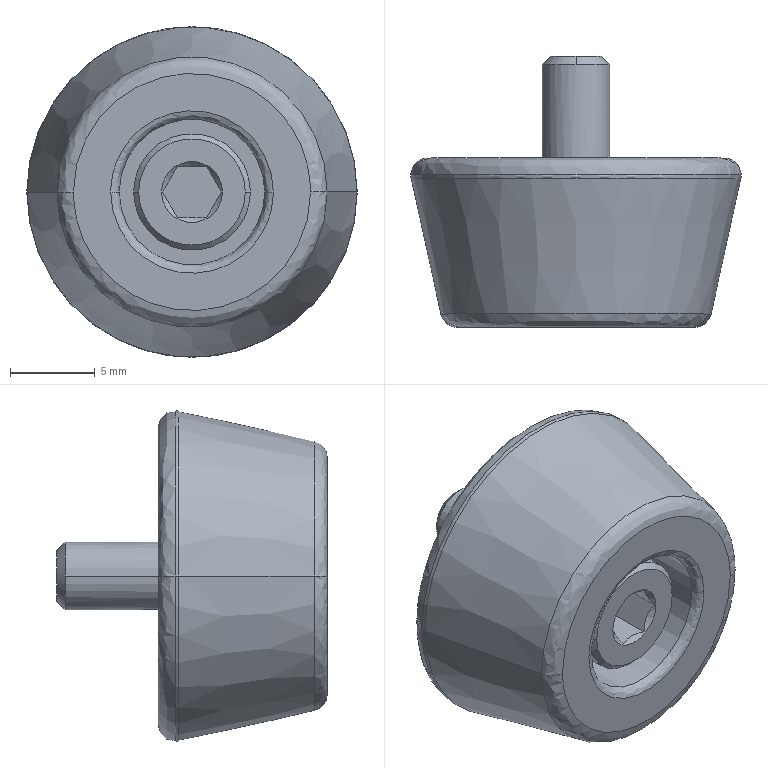Part | SolidWorks | features BaseBody 1 | 1 solid | 34 faces | box 19.513 x 16 x 19.513 mm | volume 2386 mm3 | plane 12 | spline 8 | cone 8 | cylinder 6 | commonest cylinder face diameters 4 x2 6.9 x2 8.6 x2
STEP:
#1=CARTESIAN_POINT('',(9.757,9.,0.));
#2=VERTEX_POINT('',#1);
#3=CARTESIAN_POINT('',(-9.757,9.,0.));
#4=VERTEX_POINT('',#3);
#5=CARTESIAN_POINT('',(0.,9.,0.));
#6=DIRECTION('',(0.,1.,0.));
#7=DIRECTION('',(-1.,0.,0.));
#8=AXIS2_PLACEMENT_3D('',#5,#6,#7);
#9=CIRCLE('',#8,9.757);
#10=EDGE_CURVE('',#2,#4,#9,.T.);
#11=ORIENTED_EDGE('',*,*,#10,.F.);
#12=CARTESIAN_POINT('',(9.733,8.786,0.));
#13=VERTEX_POINT('',#12);
#14=CARTESIAN_POINT('',(8.757,9.,0.));
#15=DIRECTION('',(0.,0.,-1.));
#16=DIRECTION('',(1.,0.,0.));
#17=AXIS2_PLACEMENT_3D('',#14,#15,#16);
#18=CIRCLE('',#17,1.);
#19=EDGE_CURVE('',#2,#13,#18,.T.);
#20=ORIENTED_EDGE('',*,*,#19,.T.);
#21=CARTESIAN_POINT('',(-9.733,8.786,0.));
#22=VERTEX_POINT('',#21);
#23=CARTESIAN_POINT('',(0.,8.786,0.));
#24=DIRECTION('',(0.,1.,0.));
#25=DIRECTION('',(-1.,0.,0.));
#26=AXIS2_PLACEMENT_3D('',#23,#24,#25);
#27=CIRCLE('',#26,9.733);
#28=EDGE_CURVE('',#13,#22,#27,.T.);
#29=ORIENTED_EDGE('',*,*,#28,.T.);
#30=CARTESIAN_POINT('',(-8.757,9.,0.));
#31=DIRECTION('',(0.,0.,1.));
#32=DIRECTION('',(-1.,0.,0.));
#33=AXIS2_PLACEMENT_3D('',#30,#31,#32);
#34=CIRCLE('',#33,1.);
#35=EDGE_CURVE('',#4,#22,#34,.T.);
#36=ORIENTED_EDGE('',*,*,#35,.F.);
#37=EDGE_LOOP('',(#11,#20,#29,#36));
#38=FACE_OUTER_BOUND('',#37,.T.);
#39=CARTESIAN_POINT('',(9.757,9.,0.));
#40=CARTESIAN_POINT('',(9.757,9.,-19.513));
#41=CARTESIAN_POINT('',(-9.757,9.,-19.513));
#42=CARTESIAN_POINT('',(-9.757,9.,0.));
#43=CARTESIAN_POINT('',(9.757,8.928,0.));
#44=CARTESIAN_POINT('',(9.757,8.928,-19.513));
#45=CARTESIAN_POINT('',(-9.757,8.928,-19.513));
#46=CARTESIAN_POINT('',(-9.757,8.928,0.));
#47=CARTESIAN_POINT('',(9.749,8.856,0.));
#48=CARTESIAN_POINT('',(9.749,8.856,-19.498));
#49=CARTESIAN_POINT('',(-9.749,8.856,-19.498));
#50=CARTESIAN_POINT('',(-9.749,8.856,0.));
#51=CARTESIAN_POINT('',(9.733,8.786,0.));
#52=CARTESIAN_POINT('',(9.733,8.786,-19.467));
#53=CARTESIAN_POINT('',(-9.733,8.786,-19.467));
#54=CARTESIAN_POINT('',(-9.733,8.786,0.));
#55=(BOUNDED_SURFACE()B_SPLINE_SURFACE(3,3,((#39,#40,#41,#42),(#43,#44,#45,#46),(#47,#48,#49,#50),(#51,#52,#53,#54)),.UNSPECIFIED.,.F.,.F.,.F.)B_SPLINE_SURFACE_WITH_KNOTS((4,4),(4,4),(0.,1.),(0.,1.),.UNSPECIFIED.)GEOMETRIC_REPRESENTATION_ITEM()RATIONAL_B_SPLINE_SURFACE(((1.,0.3333,0.3333,1.),(0.9961,0.332,0.332,0.9961),(0.9961,0.332,0.332,0.9961),(1.,0.3333,0.3333,1.)))REPRESENTATION_ITEM('')SURFACE());
#56=ADVANCED_FACE('',(#38),#55,.T.);
#57=CARTESIAN_POINT('',(7.977,0.7855,0.));
#58=VERTEX_POINT('',#57);
#59=CARTESIAN_POINT('',(-7.977,0.7855,0.));
#60=VERTEX_POINT('',#59);
#61=CARTESIAN_POINT('',(0.,0.7855,0.));
#62=DIRECTION('',(0.,1.,0.));
#63=DIRECTION('',(-1.,0.,0.));
#64=AXIS2_PLACEMENT_3D('',#61,#62,#63);
#65=CIRCLE('',#64,7.977);
#66=EDGE_CURVE('',#58,#60,#65,.T.);
#67=ORIENTED_EDGE('',*,*,#66,.F.);
#68=CARTESIAN_POINT('',(7.,0.,0.));
#69=VERTEX_POINT('',#68);
#70=CARTESIAN_POINT('',(7.,1.,0.));
#71=DIRECTION('',(0.,0.,-1.));
#72=DIRECTION('',(1.,0.,0.));
#73=AXIS2_PLACEMENT_3D('',#70,#71,#72);
#74=CIRCLE('',#73,1.);
#75=EDGE_CURVE('',#58,#69,#74,.T.);
#76=ORIENTED_EDGE('',*,*,#75,.T.);
#77=CARTESIAN_POINT('',(-7.,0.,0.));
#78=VERTEX_POINT('',#77);
#79=CARTESIAN_POINT('',(7.,0.,0.));
#80=CARTESIAN_POINT('',(7.,0.,-14.));
#81=CARTESIAN_POINT('',(-7.,0.,-14.));
#82=CARTESIAN_POINT('',(-7.,0.,0.));
#83=(BOUNDED_CURVE()B_SPLINE_CURVE(3,(#79,#80,#81,#82),.UNSPECIFIED.,.F.,.F.)B_SPLINE_CURVE_WITH_KNOTS((4,4),(0.,1.),.UNSPECIFIED.)CURVE()GEOMETRIC_REPRESENTATION_ITEM()RATIONAL_B_SPLINE_CURVE((1.,0.3333,0.3333,1.))REPRESENTATION_ITEM(''));
#84=EDGE_CURVE('',#69,#78,#83,.T.);
#85=ORIENTED_EDGE('',*,*,#84,.T.);
#86=CARTESIAN_POINT('',(-7.,1.,0.));
#87=DIRECTION('',(0.,0.,1.));
#88=DIRECTION('',(-1.,0.,0.));
#89=AXIS2_PLACEMENT_3D('',#86,#87,#88);
#90=CIRCLE('',#89,1.);
#91=EDGE_CURVE('',#60,#78,#90,.T.);
#92=ORIENTED_EDGE('',*,*,#91,.F.);
#93=EDGE_LOOP('',(#67,#76,#85,#92));
#94=FACE_OUTER_BOUND('',#93,.T.);
#95=CARTESIAN_POINT('',(7.977,0.7855,0.));
#96=CARTESIAN_POINT('',(7.977,0.7855,-15.953));
#97=CARTESIAN_POINT('',(-7.977,0.7855,-15.953));
#98=CARTESIAN_POINT('',(-7.977,0.7855,0.));
#99=CARTESIAN_POINT('',(7.872,0.307,0.));
#100=CARTESIAN_POINT('',(7.872,0.307,-15.743));
#101=CARTESIAN_POINT('',(-7.872,0.307,-15.743));
#102=CARTESIAN_POINT('',(-7.872,0.307,0.));
#103=CARTESIAN_POINT('',(7.49,0.,0.));
#104=CARTESIAN_POINT('',(7.49,0.,-14.98));
#105=CARTESIAN_POINT('',(-7.49,0.,-14.98));
#106=CARTESIAN_POINT('',(-7.49,0.,0.));
#107=CARTESIAN_POINT('',(7.,0.,0.));
#108=CARTESIAN_POINT('',(7.,0.,-14.));
#109=CARTESIAN_POINT('',(-7.,0.,-14.));
#110=CARTESIAN_POINT('',(-7.,0.,0.));
#111=(BOUNDED_SURFACE()B_SPLINE_SURFACE(3,3,((#95,#96,#97,#98),(#99,#100,#101,#102),(#103,#104,#105,#106),(#107,#108,#109,#110)),.UNSPECIFIED.,.F.,.F.,.F.)B_SPLINE_SURFACE_WITH_KNOTS((4,4),(4,4),(0.,1.),(0.,1.),.UNSPECIFIED.)GEOMETRIC_REPRESENTATION_ITEM()RATIONAL_B_SPLINE_SURFACE(((1.,0.3333,0.3333,1.),(0.8528,0.2843,0.2843,0.8528),(0.8528,0.2843,0.2843,0.8528),(1.,0.3333,0.3333,1.)))REPRESENTATION_ITEM('')SURFACE());
#112=ADVANCED_FACE('',(#94),#111,.T.);
#113=CARTESIAN_POINT('',(-4.8,0.,0.));
#114=VERTEX_POINT('',#113);
#115=CARTESIAN_POINT('',(4.8,0.,0.));
#116=VERTEX_POINT('',#115);
#117=CARTESIAN_POINT('',(-4.8,0.,0.));
#118=CARTESIAN_POINT('',(-4.8,0.,-9.6));
#119=CARTESIAN_POINT('',(4.8,0.,-9.6));
#120=CARTESIAN_POINT('',(4.8,0.,0.));
#121=(BOUNDED_CURVE()B_SPLINE_CURVE(3,(#117,#118,#119,#120),.UNSPECIFIED.,.F.,.F.)B_SPLINE_CURVE_WITH_KNOTS((4,4),(0.,1.),.UNSPECIFIED.)CURVE()GEOMETRIC_REPRESENTATION_ITEM()RATIONAL_B_SPLINE_CURVE((1.,0.3333,0.3333,1.))REPRESENTATION_ITEM(''));
#122=EDGE_CURVE('',#114,#116,#121,.T.);
#123=ORIENTED_EDGE('',*,*,#122,.T.);
#124=CARTESIAN_POINT('',(4.3,0.5,0.));
#125=VERTEX_POINT('',#124);
#126=CARTESIAN_POINT('',(4.8,0.5,0.));
#127=DIRECTION('',(0.,0.,-1.));
#128=DIRECTION('',(1.,0.,0.));
#129=AXIS2_PLACEMENT_3D('',#126,#127,#128);
#130=CIRCLE('',#129,0.5);
#131=EDGE_CURVE('',#116,#125,#130,.T.);
#132=ORIENTED_EDGE('',*,*,#131,.T.);
#133=CARTESIAN_POINT('',(-4.3,0.5,0.));
#134=VERTEX_POINT('',#133);
#135=CARTESIAN_POINT('',(0.,0.5,0.));
#136=DIRECTION('',(0.,1.,0.));
#137=DIRECTION('',(-1.,0.,0.));
#138=AXIS2_PLACEMENT_3D('',#135,#136,#137);
#139=CIRCLE('',#138,4.3);
#140=EDGE_CURVE('',#125,#134,#139,.T.);
#141=ORIENTED_EDGE('',*,*,#140,.T.);
#142=CARTESIAN_POINT('',(-4.8,0.5,0.));
#143=DIRECTION('',(0.,0.,1.));
#144=DIRECTION('',(-1.,0.,0.));
#145=AXIS2_PLACEMENT_3D('',#142,#143,#144);
#146=CIRCLE('',#145,0.5);
#147=EDGE_CURVE('',#114,#134,#146,.T.);
#148=ORIENTED_EDGE('',*,*,#147,.F.);
#149=EDGE_LOOP('',(#123,#132,#141,#148));
#150=FACE_OUTER_BOUND('',#149,.T.);
#151=CARTESIAN_POINT('',(4.8,0.,0.));
#152=CARTESIAN_POINT('',(4.8,0.,-9.6));
#153=CARTESIAN_POINT('',(-4.8,0.,-9.6));
#154=CARTESIAN_POINT('',(-4.8,0.,0.));
#155=CARTESIAN_POINT('',(4.507,0.,0.));
#156=CARTESIAN_POINT('',(4.507,0.,-9.014));
#157=CARTESIAN_POINT('',(-4.507,0.,-9.014));
#158=CARTESIAN_POINT('',(-4.507,0.,0.));
#159=CARTESIAN_POINT('',(4.3,0.2071,0.));
#160=CARTESIAN_POINT('',(4.3,0.2071,-8.6));
#161=CARTESIAN_POINT('',(-4.3,0.2071,-8.6));
#162=CARTESIAN_POINT('',(-4.3,0.2071,0.));
#163=CARTESIAN_POINT('',(4.3,0.5,0.));
#164=CARTESIAN_POINT('',(4.3,0.5,-8.6));
#165=CARTESIAN_POINT('',(-4.3,0.5,-8.6));
#166=CARTESIAN_POINT('',(-4.3,0.5,0.));
#167=(BOUNDED_SURFACE()B_SPLINE_SURFACE(3,3,((#151,#152,#153,#154),(#155,#156,#157,#158),(#159,#160,#161,#162),(#163,#164,#165,#166)),.UNSPECIFIED.,.F.,.F.,.F.)B_SPLINE_SURFACE_WITH_KNOTS((4,4),(4,4),(0.,1.),(0.,1.),.UNSPECIFIED.)GEOMETRIC_REPRESENTATION_ITEM()RATIONAL_B_SPLINE_SURFACE(((1.,0.3333,0.3333,1.),(0.8047,0.2682,0.2682,0.8047),(0.8047,0.2682,0.2682,0.8047),(1.,0.3333,0.3333,1.)))REPRESENTATION_ITEM('')SURFACE());
#168=ADVANCED_FACE('',(#150),#167,.T.);
#169=CARTESIAN_POINT('',(-8.757,10.,0.));
#170=VERTEX_POINT('',#169);
#171=CARTESIAN_POINT('',(8.757,10.,0.));
#172=VERTEX_POINT('',#171);
#173=CARTESIAN_POINT('',(-8.757,10.,0.));
#174=CARTESIAN_POINT('',(-8.757,10.,-17.513));
#175=CARTESIAN_POINT('',(8.757,10.,-17.513));
#176=CARTESIAN_POINT('',(8.757,10.,0.));
#177=(BOUNDED_CURVE()B_SPLINE_CURVE(3,(#173,#174,#175,#176),.UNSPECIFIED.,.F.,.F.)B_SPLINE_CURVE_WITH_KNOTS((4,4),(0.,1.),.UNSPECIFIED.)CURVE()GEOMETRIC_REPRESENTATION_ITEM()RATIONAL_B_SPLINE_CURVE((1.,0.3333,0.3333,1.))REPRESENTATION_ITEM(''));
#178=EDGE_CURVE('',#170,#172,#177,.T.);
#179=ORIENTED_EDGE('',*,*,#178,.T.);
#180=CARTESIAN_POINT('',(8.757,9.,0.));
#181=DIRECTION('',(0.,0.,-1.));
#182=DIRECTION('',(1.,0.,0.));
#183=AXIS2_PLACEMENT_3D('',#180,#181,#182);
#184=CIRCLE('',#183,1.);
#185=EDGE_CURVE('',#172,#2,#184,.T.);
#186=ORIENTED_EDGE('',*,*,#185,.T.);
#187=ORIENTED_EDGE('',*,*,#10,.T.);
#188=CARTESIAN_POINT('',(-8.757,9.,0.));
#189=DIRECTION('',(0.,0.,1.));
#190=DIRECTION('',(-1.,0.,0.));
#191=AXIS2_PLACEMENT_3D('',#188,#189,#190);
#192=CIRCLE('',#191,1.);
#193=EDGE_CURVE('',#170,#4,#192,.T.);
#194=ORIENTED_EDGE('',*,*,#193,.F.);
#195=EDGE_LOOP('',(#179,#186,#187,#194));
#196=FACE_OUTER_BOUND('',#195,.T.);
#197=CARTESIAN_POINT('',(8.757,10.,0.));
#198=CARTESIAN_POINT('',(8.757,10.,-17.513));
#199=CARTESIAN_POINT('',(-8.757,10.,-17.513));
#200=CARTESIAN_POINT('',(-8.757,10.,0.));
#201=CARTESIAN_POINT('',(9.342,10.,0.));
#202=CARTESIAN_POINT('',(9.342,10.,-18.685));
#203=CARTESIAN_POINT('',(-9.342,10.,-18.685));
#204=CARTESIAN_POINT('',(-9.342,10.,0.));
#205=CARTESIAN_POINT('',(9.757,9.586,0.));
#206=CARTESIAN_POINT('',(9.757,9.586,-19.513));
#207=CARTESIAN_POINT('',(-9.757,9.586,-19.513));
#208=CARTESIAN_POINT('',(-9.757,9.586,0.));
#209=CARTESIAN_POINT('',(9.757,9.,0.));
#210=CARTESIAN_POINT('',(9.757,9.,-19.513));
#211=CARTESIAN_POINT('',(-9.757,9.,-19.513));
#212=CARTESIAN_POINT('',(-9.757,9.,0.));
#213=(BOUNDED_SURFACE()B_SPLINE_SURFACE(3,3,((#197,#198,#199,#200),(#201,#202,#203,#204),(#205,#206,#207,#208),(#209,#210,#211,#212)),.UNSPECIFIED.,.F.,.F.,.F.)B_SPLINE_SURFACE_WITH_KNOTS((4,4),(4,4),(0.,1.),(0.,1.),.UNSPECIFIED.)GEOMETRIC_REPRESENTATION_ITEM()RATIONAL_B_SPLINE_SURFACE(((1.,0.3333,0.3333,1.),(0.8047,0.2682,0.2682,0.8047),(0.8047,0.2682,0.2682,0.8047),(1.,0.3333,0.3333,1.)))REPRESENTATION_ITEM('')SURFACE());
#214=ADVANCED_FACE('',(#196),#213,.T.);
#215=ORIENTED_EDGE('',*,*,#185,.F.);
#216=CARTESIAN_POINT('',(8.757,10.,0.));
#217=CARTESIAN_POINT('',(8.757,10.,17.513));
#218=CARTESIAN_POINT('',(-8.757,10.,17.513));
#219=CARTESIAN_POINT('',(-8.757,10.,0.));
#220=(BOUNDED_CURVE()B_SPLINE_CURVE(3,(#216,#217,#218,#219),.UNSPECIFIED.,.F.,.T.)B_SPLINE_CURVE_WITH_KNOTS((4,4),(0.,1.),.UNSPECIFIED.)CURVE()GEOMETRIC_REPRESENTATION_ITEM()RATIONAL_B_SPLINE_CURVE((1.,0.3333,0.3333,1.))REPRESENTATION_ITEM(''));
#221=EDGE_CURVE('',#172,#170,#220,.T.);
#222=ORIENTED_EDGE('',*,*,#221,.T.);
#223=ORIENTED_EDGE('',*,*,#193,.T.);
#224=CARTESIAN_POINT('',(0.,9.,0.));
#225=DIRECTION('',(0.,1.,0.));
#226=DIRECTION('',(-1.,0.,0.));
#227=AXIS2_PLACEMENT_3D('',#224,#225,#226);
#228=CIRCLE('',#227,9.757);
#229=EDGE_CURVE('',#4,#2,#228,.T.);
#230=ORIENTED_EDGE('',*,*,#229,.T.);
#231=EDGE_LOOP('',(#215,#222,#223,#230));
#232=FACE_OUTER_BOUND('',#231,.T.);
#233=CARTESIAN_POINT('',(-8.757,10.,0.));
#234=CARTESIAN_POINT('',(-8.757,10.,17.513));
#235=CARTESIAN_POINT('',(8.757,10.,17.513));
#236=CARTESIAN_POINT('',(8.757,10.,0.));
#237=CARTESIAN_POINT('',(-9.342,10.,0.));
#238=CARTESIAN_POINT('',(-9.342,10.,18.685));
#239=CARTESIAN_POINT('',(9.342,10.,18.685));
#240=CARTESIAN_POINT('',(9.342,10.,0.));
#241=CARTESIAN_POINT('',(-9.757,9.586,0.));
#242=CARTESIAN_POINT('',(-9.757,9.586,19.513));
#243=CARTESIAN_POINT('',(9.757,9.586,19.513));
#244=CARTESIAN_POINT('',(9.757,9.586,0.));
#245=CARTESIAN_POINT('',(-9.757,9.,0.));
#246=CARTESIAN_POINT('',(-9.757,9.,19.513));
#247=CARTESIAN_POINT('',(9.757,9.,19.513));
#248=CARTESIAN_POINT('',(9.757,9.,0.));
#249=(BOUNDED_SURFACE()B_SPLINE_SURFACE(3,3,((#233,#234,#235,#236),(#237,#238,#239,#240),(#241,#242,#243,#244),(#245,#246,#247,#248)),.UNSPECIFIED.,.F.,.F.,.F.)B_SPLINE_SURFACE_WITH_KNOTS((4,4),(4,4),(0.,1.),(0.,1.),.UNSPECIFIED.)GEOMETRIC_REPRESENTATION_ITEM()RATIONAL_B_SPLINE_SURFACE(((1.,0.3333,0.3333,1.),(0.8047,0.2682,0.2682,0.8047),(0.8047,0.2682,0.2682,0.8047),(1.,0.3333,0.3333,1.)))REPRESENTATION_ITEM('')SURFACE());
#250=ADVANCED_FACE('',(#232),#249,.T.);
#251=CARTESIAN_POINT('',(-2.,10.,0.));
#252=VERTEX_POINT('',#251);
#253=CARTESIAN_POINT('',(2.,10.,0.));
#254=VERTEX_POINT('',#253);
#255=CARTESIAN_POINT('',(0.,10.,0.));
#256=DIRECTION('',(0.,1.,0.));
#257=DIRECTION('',(-1.,0.,0.));
#258=AXIS2_PLACEMENT_3D('',#255,#256,#257);
#259=CIRCLE('',#258,2.);
#260=EDGE_CURVE('',#252,#254,#259,.T.);
#261=ORIENTED_EDGE('',*,*,#260,.T.);
#262=CARTESIAN_POINT('',(2.,15.5,0.));
#263=VERTEX_POINT('',#262);
#264=CARTESIAN_POINT('',(2.,16.,0.));
#265=DIRECTION('',(0.,1.,0.));
#266=VECTOR('',#265,1000.);
#267=LINE('',#264,#266);
#268=EDGE_CURVE('',#254,#263,#267,.T.);
#269=ORIENTED_EDGE('',*,*,#268,.T.);
#270=CARTESIAN_POINT('',(0.,15.5,2.));
#271=VERTEX_POINT('',#270);
#272=CARTESIAN_POINT('',(0.,15.5,0.));
#273=DIRECTION('',(0.,-1.,0.));
#274=DIRECTION('',(-1.,0.,0.));
#275=AXIS2_PLACEMENT_3D('',#272,#273,#274);
#276=CIRCLE('',#275,2.);
#277=EDGE_CURVE('',#263,#271,#276,.T.);
#278=ORIENTED_EDGE('',*,*,#277,.T.);
#279=CARTESIAN_POINT('',(-2.,15.5,0.));
#280=VERTEX_POINT('',#279);
#281=CARTESIAN_POINT('',(0.,15.5,0.));
#282=DIRECTION('',(0.,-1.,0.));
#283=DIRECTION('',(-1.,0.,0.));
#284=AXIS2_PLACEMENT_3D('',#281,#282,#283);
#285=CIRCLE('',#284,2.);
#286=EDGE_CURVE('',#271,#280,#285,.T.);
#287=ORIENTED_EDGE('',*,*,#286,.T.);
#288=CARTESIAN_POINT('',(-2.,16.,0.));
#289=DIRECTION('',(0.,1.,0.));
#290=VECTOR('',#289,1000.);
#291=LINE('',#288,#290);
#292=EDGE_CURVE('',#252,#280,#291,.T.);
#293=ORIENTED_EDGE('',*,*,#292,.F.);
#294=EDGE_LOOP('',(#261,#269,#278,#287,#293));
#295=FACE_OUTER_BOUND('',#294,.T.);
#296=CARTESIAN_POINT('',(0.,16.,0.));
#297=DIRECTION('',(0.,1.,0.));
#298=DIRECTION('',(-1.,0.,0.));
#299=AXIS2_PLACEMENT_3D('',#296,#297,#298);
#300=CYLINDRICAL_SURFACE('',#299,2.);
#301=ADVANCED_FACE('',(#295),#300,.T.);
#302=CARTESIAN_POINT('',(0.,0.7855,0.));
#303=DIRECTION('',(0.,1.,0.));
#304=DIRECTION('',(-1.,0.,0.));
#305=AXIS2_PLACEMENT_3D('',#302,#303,#304);
#306=CIRCLE('',#305,7.977);
#307=EDGE_CURVE('',#60,#58,#306,.T.);
#308=ORIENTED_EDGE('',*,*,#307,.T.);
#309=CARTESIAN_POINT('',(9.733,8.786,0.));
#310=DIRECTION('',(0.2145,0.9767,0.));
#311=VECTOR('',#310,1000.);
#312=LINE('',#309,#311);
#313=EDGE_CURVE('',#58,#13,#312,.T.);
#314=ORIENTED_EDGE('',*,*,#313,.T.);
#315=CARTESIAN_POINT('',(0.,8.786,0.));
#316=DIRECTION('',(0.,1.,0.));
#317=DIRECTION('',(-1.,0.,0.));
#318=AXIS2_PLACEMENT_3D('',#315,#316,#317);
#319=CIRCLE('',#318,9.733);
#320=EDGE_CURVE('',#22,#13,#319,.T.);
#321=ORIENTED_EDGE('',*,*,#320,.F.);
#322=CARTESIAN_POINT('',(-9.733,8.786,0.));
#323=DIRECTION('',(-0.2145,0.9767,0.));
#324=VECTOR('',#323,1000.);
#325=LINE('',#322,#324);
#326=EDGE_CURVE('',#60,#22,#325,.T.);
#327=ORIENTED_EDGE('',*,*,#326,.F.);
#328=EDGE_LOOP('',(#308,#314,#321,#327));
#329=FACE_OUTER_BOUND('',#328,.T.);
#330=CARTESIAN_POINT('',(0.,8.786,0.));
#331=DIRECTION('',(0.,1.,0.));
#332=DIRECTION('',(-1.,0.,0.));
#333=AXIS2_PLACEMENT_3D('',#330,#331,#332);
#334=CONICAL_SURFACE('',#333,9.733,0.2161);
#335=ADVANCED_FACE('',(#329),#334,.T.);
#336=CARTESIAN_POINT('',(0.,16.,-1.5));
#337=VERTEX_POINT('',#336);
#338=CARTESIAN_POINT('',(0.,16.,1.5));
#339=VERTEX_POINT('',#338);
#340=CARTESIAN_POINT('',(0.,16.,0.));
#341=DIRECTION('',(0.,-1.,0.));
#342=DIRECTION('',(0.,0.,-1.));
#343=AXIS2_PLACEMENT_3D('',#340,#341,#342);
#344=CIRCLE('',#343,1.5);
#345=EDGE_CURVE('',#337,#339,#344,.T.);
#346=ORIENTED_EDGE('',*,*,#345,.T.);
#347=CARTESIAN_POINT('',(0.,15.5,2.));
#348=DIRECTION('',(0.,-0.7071,0.7071));
#349=VECTOR('',#348,1000.);
#350=LINE('',#347,#349);
#351=EDGE_CURVE('',#339,#271,#350,.T.);
#352=ORIENTED_EDGE('',*,*,#351,.T.);
#353=ORIENTED_EDGE('',*,*,#277,.F.);
#354=CARTESIAN_POINT('',(0.,15.5,-2.));
#355=VERTEX_POINT('',#354);
#356=CARTESIAN_POINT('',(0.,15.5,0.));
#357=DIRECTION('',(0.,-1.,0.));
#358=DIRECTION('',(-1.,0.,0.));
#359=AXIS2_PLACEMENT_3D('',#356,#357,#358);
#360=CIRCLE('',#359,2.);
#361=EDGE_CURVE('',#355,#263,#360,.T.);
#362=ORIENTED_EDGE('',*,*,#361,.F.);
#363=CARTESIAN_POINT('',(0.,15.5,-2.));
#364=DIRECTION('',(0.,-0.7071,-0.7071));
#365=VECTOR('',#364,1000.);
#366=LINE('',#363,#365);
#367=EDGE_CURVE('',#337,#355,#366,.T.);
#368=ORIENTED_EDGE('',*,*,#367,.F.);
#369=EDGE_LOOP('',(#346,#352,#353,#362,#368));
#370=FACE_OUTER_BOUND('',#369,.T.);
#371=CARTESIAN_POINT('',(0.,15.5,0.));
#372=DIRECTION('',(0.,-1.,0.));
#373=DIRECTION('',(0.,0.,-1.));
#374=AXIS2_PLACEMENT_3D('',#371,#372,#373);
#375=CONICAL_SURFACE('',#374,2.,0.7854);
#376=ADVANCED_FACE('',(#370),#375,.T.);
#377=ORIENTED_EDGE('',*,*,#140,.F.);
#378=CARTESIAN_POINT('',(4.3,5.,0.));
#379=VERTEX_POINT('',#378);
#380=CARTESIAN_POINT('',(4.3,16.,0.));
#381=DIRECTION('',(0.,1.,0.));
#382=VECTOR('',#381,1000.);
#383=LINE('',#380,#382);
#384=EDGE_CURVE('',#125,#379,#383,.T.);
#385=ORIENTED_EDGE('',*,*,#384,.T.);
#386=CARTESIAN_POINT('',(-4.3,5.,0.));
#387=VERTEX_POINT('',#386);
#388=CARTESIAN_POINT('',(0.,5.,0.));
#389=DIRECTION('',(0.,-1.,0.));
#390=DIRECTION('',(-1.,0.,0.));
#391=AXIS2_PLACEMENT_3D('',#388,#389,#390);
#392=CIRCLE('',#391,4.3);
#393=EDGE_CURVE('',#387,#379,#392,.T.);
#394=ORIENTED_EDGE('',*,*,#393,.F.);
#395=CARTESIAN_POINT('',(-4.3,16.,0.));
#396=DIRECTION('',(0.,1.,0.));
#397=VECTOR('',#396,1000.);
#398=LINE('',#395,#397);
#399=EDGE_CURVE('',#134,#387,#398,.T.);
#400=ORIENTED_EDGE('',*,*,#399,.F.);
#401=EDGE_LOOP('',(#377,#385,#394,#400));
#402=FACE_OUTER_BOUND('',#401,.T.);
#403=CARTESIAN_POINT('',(0.,16.,0.));
#404=DIRECTION('',(0.,1.,0.));
#405=DIRECTION('',(-1.,0.,0.));
#406=AXIS2_PLACEMENT_3D('',#403,#404,#405);
#407=CYLINDRICAL_SURFACE('',#406,4.3);
#408=ADVANCED_FACE('',(#402),#407,.F.);
#409=CARTESIAN_POINT('',(-3.45,1.3,0.));
#410=VERTEX_POINT('',#409);
#411=CARTESIAN_POINT('',(3.45,1.3,0.));
#412=VERTEX_POINT('',#411);
#413=CARTESIAN_POINT('',(0.,1.3,0.));
#414=DIRECTION('',(0.,1.,0.));
#415=DIRECTION('',(-1.,0.,0.));
#416=AXIS2_PLACEMENT_3D('',#413,#414,#415);
#417=CIRCLE('',#416,3.45);
#418=EDGE_CURVE('',#410,#412,#417,.T.);
#419=ORIENTED_EDGE('',*,*,#418,.T.);
#420=CARTESIAN_POINT('',(3.45,5.,0.));
#421=VERTEX_POINT('',#420);
#422=CARTESIAN_POINT('',(3.45,16.,0.));
#423=DIRECTION('',(0.,1.,0.));
#424=VECTOR('',#423,1000.);
#425=LINE('',#422,#424);
#426=EDGE_CURVE('',#412,#421,#425,.T.);
#427=ORIENTED_EDGE('',*,*,#426,.T.);
#428=CARTESIAN_POINT('',(-3.45,5.,0.));
#429=VERTEX_POINT('',#428);
#430=CARTESIAN_POINT('',(0.,5.,0.));
#431=DIRECTION('',(0.,-1.,0.));
#432=DIRECTION('',(-1.,0.,0.));
#433=AXIS2_PLACEMENT_3D('',#430,#431,#432);
#434=CIRCLE('',#433,3.45);
#435=EDGE_CURVE('',#421,#429,#434,.T.);
#436=ORIENTED_EDGE('',*,*,#435,.T.);
#437=CARTESIAN_POINT('',(-3.45,16.,0.));
#438=DIRECTION('',(0.,1.,0.));
#439=VECTOR('',#438,1000.);
#440=LINE('',#437,#439);
#441=EDGE_CURVE('',#410,#429,#440,.T.);
#442=ORIENTED_EDGE('',*,*,#441,.F.);
#443=EDGE_LOOP('',(#419,#427,#436,#442));
#444=FACE_OUTER_BOUND('',#443,.T.);
#445=CARTESIAN_POINT('',(0.,16.,0.));
#446=DIRECTION('',(0.,1.,0.));
#447=DIRECTION('',(-1.,0.,0.));
#448=AXIS2_PLACEMENT_3D('',#445,#446,#447);
#449=CYLINDRICAL_SURFACE('',#448,3.45);
#450=ADVANCED_FACE('',(#444),#449,.T.);
#451=CARTESIAN_POINT('',(-3.15,1.,0.));
#452=VERTEX_POINT('',#451);
#453=CARTESIAN_POINT('',(3.15,1.,0.));
#454=VERTEX_POINT('',#453);
#455=CARTESIAN_POINT('',(0.,1.,0.));
#456=DIRECTION('',(0.,1.,0.));
#457=DIRECTION('',(-1.,0.,0.));
#458=AXIS2_PLACEMENT_3D('',#455,#456,#457);
#459=CIRCLE('',#458,3.15);
#460=EDGE_CURVE('',#452,#454,#459,.T.);
#461=ORIENTED_EDGE('',*,*,#460,.T.);
#462=CARTESIAN_POINT('',(3.45,1.3,0.));
#463=DIRECTION('',(0.7071,0.7071,0.));
#464=VECTOR('',#463,1000.);
#465=LINE('',#462,#464);
#466=EDGE_CURVE('',#454,#412,#465,.T.);
#467=ORIENTED_EDGE('',*,*,#466,.T.);
#468=ORIENTED_EDGE('',*,*,#418,.F.);
#469=CARTESIAN_POINT('',(-3.45,1.3,0.));
#470=DIRECTION('',(-0.7071,0.7071,0.));
#471=VECTOR('',#470,1000.);
#472=LINE('',#469,#471);
#473=EDGE_CURVE('',#452,#410,#472,.T.);
#474=ORIENTED_EDGE('',*,*,#473,.F.);
#475=EDGE_LOOP('',(#461,#467,#468,#474));
#476=FACE_OUTER_BOUND('',#475,.T.);
#477=CARTESIAN_POINT('',(0.,1.3,0.));
#478=DIRECTION('',(0.,1.,0.));
#479=DIRECTION('',(-1.,0.,0.));
#480=AXIS2_PLACEMENT_3D('',#477,#478,#479);
#481=CONICAL_SURFACE('',#480,3.45,0.7854);
#482=ADVANCED_FACE('',(#476),#481,.T.);
#483=CARTESIAN_POINT('',(-1.732,1.068,0.));
#484=VERTEX_POINT('',#483);
#485=CARTESIAN_POINT('',(-0.866,1.068,-1.5));
#486=VERTEX_POINT('',#485);
#487=CARTESIAN_POINT('',(-1.732,1.068,0.));
#488=CARTESIAN_POINT('',(-1.664,1.136,-0.1172));
#489=CARTESIAN_POINT('',(-1.595,1.193,-0.237));
#490=CARTESIAN_POINT('',(-1.452,1.275,-0.4853));
#491=CARTESIAN_POINT('',(-1.376,1.3,-0.6163));
#492=CARTESIAN_POINT('',(-1.149,1.301,-1.009));
#493=CARTESIAN_POINT('',(-1.002,1.204,-1.264));
#494=CARTESIAN_POINT('',(-0.866,1.068,-1.5));
#495=B_SPLINE_CURVE_WITH_KNOTS('',3,(#487,#488,#489,#490,#491,#492,#493,#494),.UNSPECIFIED.,.F.,.F.,(4,2,2,4),(0.,0.0004473,0.0008946,0.001789),.UNSPECIFIED.);
#496=EDGE_CURVE('',#484,#486,#495,.T.);
#497=ORIENTED_EDGE('',*,*,#496,.F.);
#498=CARTESIAN_POINT('',(-1.8,1.,0.));
#499=VERTEX_POINT('',#498);
#500=CARTESIAN_POINT('',(-1.8,1.,0.));
#501=DIRECTION('',(-0.7071,-0.7071,0.));
#502=VECTOR('',#501,1000.);
#503=LINE('',#500,#502);
#504=EDGE_CURVE('',#484,#499,#503,.T.);
#505=ORIENTED_EDGE('',*,*,#504,.T.);
#506=CARTESIAN_POINT('',(1.8,1.,0.));
#507=VERTEX_POINT('',#506);
#508=CARTESIAN_POINT('',(0.,1.,0.));
#509=DIRECTION('',(0.,-1.,0.));
#510=DIRECTION('',(1.,0.,0.));
#511=AXIS2_PLACEMENT_3D('',#508,#509,#510);
#512=CIRCLE('',#511,1.8);
#513=EDGE_CURVE('',#499,#507,#512,.T.);
#514=ORIENTED_EDGE('',*,*,#513,.T.);
#515=CARTESIAN_POINT('',(1.732,1.068,0.));
#516=VERTEX_POINT('',#515);
#517=CARTESIAN_POINT('',(1.8,1.,0.));
#518=DIRECTION('',(0.7071,-0.7071,0.));
#519=VECTOR('',#518,1000.);
#520=LINE('',#517,#519);
#521=EDGE_CURVE('',#516,#507,#520,.T.);
#522=ORIENTED_EDGE('',*,*,#521,.F.);
#523=CARTESIAN_POINT('',(0.866,1.068,-1.5));
#524=VERTEX_POINT('',#523);
#525=CARTESIAN_POINT('',(0.866,1.068,-1.5));
#526=CARTESIAN_POINT('',(0.9337,1.136,-1.383));
#527=CARTESIAN_POINT('',(1.003,1.193,-1.263));
#528=CARTESIAN_POINT('',(1.146,1.275,-1.015));
#529=CARTESIAN_POINT('',(1.222,1.3,-0.8837));
#530=CARTESIAN_POINT('',(1.449,1.301,-0.4909));
#531=CARTESIAN_POINT('',(1.596,1.204,-0.2358));
#532=CARTESIAN_POINT('',(1.732,1.068,0.));
#533=B_SPLINE_CURVE_WITH_KNOTS('',3,(#525,#526,#527,#528,#529,#530,#531,#532),.UNSPECIFIED.,.F.,.F.,(4,2,2,4),(0.,0.0004473,0.0008946,0.001789),.UNSPECIFIED.);
#534=EDGE_CURVE('',#524,#516,#533,.T.);
#535=ORIENTED_EDGE('',*,*,#534,.F.);
#536=CARTESIAN_POINT('',(-0.866,1.068,-1.5));
#537=CARTESIAN_POINT('',(-0.7307,1.136,-1.5));
#538=CARTESIAN_POINT('',(-0.5923,1.193,-1.5));
#539=CARTESIAN_POINT('',(-0.3056,1.275,-1.5));
#540=CARTESIAN_POINT('',(-0.1544,1.3,-1.5));
#541=CARTESIAN_POINT('',(0.2992,1.301,-1.5));
#542=CARTESIAN_POINT('',(0.5938,1.204,-1.5));
#543=CARTESIAN_POINT('',(0.866,1.068,-1.5));
#544=B_SPLINE_CURVE_WITH_KNOTS('',3,(#536,#537,#538,#539,#540,#541,#542,#543),.UNSPECIFIED.,.F.,.F.,(4,2,2,4),(0.,0.0004473,0.0008946,0.001789),.UNSPECIFIED.);
#545=EDGE_CURVE('',#486,#524,#544,.T.);
#546=ORIENTED_EDGE('',*,*,#545,.F.);
#547=EDGE_LOOP('',(#497,#505,#514,#522,#535,#546));
#548=FACE_OUTER_BOUND('',#547,.T.);
#549=CARTESIAN_POINT('',(0.,1.,0.));
#550=DIRECTION('',(0.,-1.,0.));
#551=DIRECTION('',(1.,0.,0.));
#552=AXIS2_PLACEMENT_3D('',#549,#550,#551);
#553=CONICAL_SURFACE('',#552,1.8,0.7854);
#554=ADVANCED_FACE('',(#548),#553,.F.);
#555=ORIENTED_EDGE('',*,*,#178,.F.);
#556=ORIENTED_EDGE('',*,*,#221,.F.);
#557=EDGE_LOOP('',(#555,#556));
#558=FACE_OUTER_BOUND('',#557,.T.);
#559=ORIENTED_EDGE('',*,*,#260,.F.);
#560=CARTESIAN_POINT('',(0.,10.,0.));
#561=DIRECTION('',(0.,1.,0.));
#562=DIRECTION('',(-1.,0.,0.));
#563=AXIS2_PLACEMENT_3D('',#560,#561,#562);
#564=CIRCLE('',#563,2.);
#565=EDGE_CURVE('',#254,#252,#564,.T.);
#566=ORIENTED_EDGE('',*,*,#565,.F.);
#567=EDGE_LOOP('',(#559,#566));
#568=FACE_BOUND('',#567,.T.);
#569=CARTESIAN_POINT('',(8.757,10.,0.));
#570=DIRECTION('',(0.,-1.,0.));
#571=DIRECTION('',(1.,0.,0.));
#572=AXIS2_PLACEMENT_3D('',#569,#570,#571);
#573=PLANE('',#572);
#574=ADVANCED_FACE('',(#558,#568),#573,.F.);
#575=ORIENTED_EDGE('',*,*,#19,.F.);
#576=ORIENTED_EDGE('',*,*,#229,.F.);
#577=ORIENTED_EDGE('',*,*,#35,.T.);
#578=ORIENTED_EDGE('',*,*,#320,.T.);
#579=EDGE_LOOP('',(#575,#576,#577,#578));
#580=FACE_OUTER_BOUND('',#579,.T.);
#581=CARTESIAN_POINT('',(-9.757,9.,0.));
#582=CARTESIAN_POINT('',(-9.757,9.,19.513));
#583=CARTESIAN_POINT('',(9.757,9.,19.513));
#584=CARTESIAN_POINT('',(9.757,9.,0.));
#585=CARTESIAN_POINT('',(-9.757,8.928,0.));
#586=CARTESIAN_POINT('',(-9.757,8.928,19.513));
#587=CARTESIAN_POINT('',(9.757,8.928,19.513));
#588=CARTESIAN_POINT('',(9.757,8.928,0.));
#589=CARTESIAN_POINT('',(-9.749,8.856,0.));
#590=CARTESIAN_POINT('',(-9.749,8.856,19.498));
#591=CARTESIAN_POINT('',(9.749,8.856,19.498));
#592=CARTESIAN_POINT('',(9.749,8.856,0.));
#593=CARTESIAN_POINT('',(-9.733,8.786,0.));
#594=CARTESIAN_POINT('',(-9.733,8.786,19.467));
#595=CARTESIAN_POINT('',(9.733,8.786,19.467));
#596=CARTESIAN_POINT('',(9.733,8.786,0.));
#597=(BOUNDED_SURFACE()B_SPLINE_SURFACE(3,3,((#581,#582,#583,#584),(#585,#586,#587,#588),(#589,#590,#591,#592),(#593,#594,#595,#596)),.UNSPECIFIED.,.F.,.F.,.F.)B_SPLINE_SURFACE_WITH_KNOTS((4,4),(4,4),(0.,1.),(0.,1.),.UNSPECIFIED.)GEOMETRIC_REPRESENTATION_ITEM()RATIONAL_B_SPLINE_SURFACE(((1.,0.3333,0.3333,1.),(0.9961,0.332,0.332,0.9961),(0.9961,0.332,0.332,0.9961),(1.,0.3333,0.3333,1.)))REPRESENTATION_ITEM('')SURFACE());
#598=ADVANCED_FACE('',(#580),#597,.T.);
#599=ORIENTED_EDGE('',*,*,#268,.F.);
#600=ORIENTED_EDGE('',*,*,#565,.T.);
#601=ORIENTED_EDGE('',*,*,#292,.T.);
#602=CARTESIAN_POINT('',(0.,15.5,0.));
#603=DIRECTION('',(0.,-1.,0.));
#604=DIRECTION('',(-1.,0.,0.));
#605=AXIS2_PLACEMENT_3D('',#602,#603,#604);
#606=CIRCLE('',#605,2.);
#607=EDGE_CURVE('',#280,#355,#606,.T.);
#608=ORIENTED_EDGE('',*,*,#607,.T.);
#609=ORIENTED_EDGE('',*,*,#361,.T.);
#610=EDGE_LOOP('',(#599,#600,#601,#608,#609));
#611=FACE_OUTER_BOUND('',#610,.T.);
#612=CARTESIAN_POINT('',(0.,16.,0.));
#613=DIRECTION('',(0.,1.,0.));
#614=DIRECTION('',(-1.,0.,0.));
#615=AXIS2_PLACEMENT_3D('',#612,#613,#614);
#616=CYLINDRICAL_SURFACE('',#615,2.);
#617=ADVANCED_FACE('',(#611),#616,.T.);
#618=ORIENTED_EDGE('',*,*,#313,.F.);
#619=ORIENTED_EDGE('',*,*,#66,.T.);
#620=ORIENTED_EDGE('',*,*,#326,.T.);
#621=ORIENTED_EDGE('',*,*,#28,.F.);
#622=EDGE_LOOP('',(#618,#619,#620,#621));
#623=FACE_OUTER_BOUND('',#622,.T.);
#624=CARTESIAN_POINT('',(0.,8.786,0.));
#625=DIRECTION('',(0.,1.,0.));
#626=DIRECTION('',(-1.,0.,0.));
#627=AXIS2_PLACEMENT_3D('',#624,#625,#626);
#628=CONICAL_SURFACE('',#627,9.733,0.2161);
#629=ADVANCED_FACE('',(#623),#628,.T.);
#630=ORIENTED_EDGE('',*,*,#351,.F.);
#631=CARTESIAN_POINT('',(0.,16.,0.));
#632=DIRECTION('',(0.,-1.,0.));
#633=DIRECTION('',(0.,0.,-1.));
#634=AXIS2_PLACEMENT_3D('',#631,#632,#633);
#635=CIRCLE('',#634,1.5);
#636=EDGE_CURVE('',#339,#337,#635,.T.);
#637=ORIENTED_EDGE('',*,*,#636,.T.);
#638=ORIENTED_EDGE('',*,*,#367,.T.);
#639=ORIENTED_EDGE('',*,*,#607,.F.);
#640=ORIENTED_EDGE('',*,*,#286,.F.);
#641=EDGE_LOOP('',(#630,#637,#638,#639,#640));
#642=FACE_OUTER_BOUND('',#641,.T.);
#643=CARTESIAN_POINT('',(0.,15.5,0.));
#644=DIRECTION('',(0.,-1.,0.));
#645=DIRECTION('',(0.,0.,-1.));
#646=AXIS2_PLACEMENT_3D('',#643,#644,#645);
#647=CONICAL_SURFACE('',#646,2.,0.7854);
#648=ADVANCED_FACE('',(#642),#647,.T.);
#649=ORIENTED_EDGE('',*,*,#75,.F.);
#650=ORIENTED_EDGE('',*,*,#307,.F.);
#651=ORIENTED_EDGE('',*,*,#91,.T.);
#652=CARTESIAN_POINT('',(-7.,0.,0.));
#653=CARTESIAN_POINT('',(-7.,0.,14.));
#654=CARTESIAN_POINT('',(7.,0.,14.));
#655=CARTESIAN_POINT('',(7.,0.,0.));
#656=(BOUNDED_CURVE()B_SPLINE_CURVE(3,(#652,#653,#654,#655),.UNSPECIFIED.,.F.,.F.)B_SPLINE_CURVE_WITH_KNOTS((4,4),(0.,1.),.UNSPECIFIED.)CURVE()GEOMETRIC_REPRESENTATION_ITEM()RATIONAL_B_SPLINE_CURVE((1.,0.3333,0.3333,1.))REPRESENTATION_ITEM(''));
#657=EDGE_CURVE('',#78,#69,#656,.T.);
#658=ORIENTED_EDGE('',*,*,#657,.T.);
#659=EDGE_LOOP('',(#649,#650,#651,#658));
#660=FACE_OUTER_BOUND('',#659,.T.);
#661=CARTESIAN_POINT('',(-7.977,0.7855,0.));
#662=CARTESIAN_POINT('',(-7.977,0.7855,15.953));
#663=CARTESIAN_POINT('',(7.977,0.7855,15.953));
#664=CARTESIAN_POINT('',(7.977,0.7855,0.));
#665=CARTESIAN_POINT('',(-7.872,0.307,0.));
#666=CARTESIAN_POINT('',(-7.872,0.307,15.743));
#667=CARTESIAN_POINT('',(7.872,0.307,15.743));
#668=CARTESIAN_POINT('',(7.872,0.307,0.));
#669=CARTESIAN_POINT('',(-7.49,0.,0.));
#670=CARTESIAN_POINT('',(-7.49,0.,14.98));
#671=CARTESIAN_POINT('',(7.49,0.,14.98));
#672=CARTESIAN_POINT('',(7.49,0.,0.));
#673=CARTESIAN_POINT('',(-7.,0.,0.));
#674=CARTESIAN_POINT('',(-7.,0.,14.));
#675=CARTESIAN_POINT('',(7.,0.,14.));
#676=CARTESIAN_POINT('',(7.,0.,0.));
#677=(BOUNDED_SURFACE()B_SPLINE_SURFACE(3,3,((#661,#662,#663,#664),(#665,#666,#667,#668),(#669,#670,#671,#672),(#673,#674,#675,#676)),.UNSPECIFIED.,.F.,.F.,.F.)B_SPLINE_SURFACE_WITH_KNOTS((4,4),(4,4),(0.,1.),(0.,1.),.UNSPECIFIED.)GEOMETRIC_REPRESENTATION_ITEM()RATIONAL_B_SPLINE_SURFACE(((1.,0.3333,0.3333,1.),(0.8528,0.2843,0.2843,0.8528),(0.8528,0.2843,0.2843,0.8528),(1.,0.3333,0.3333,1.)))REPRESENTATION_ITEM('')SURFACE());
#678=ADVANCED_FACE('',(#660),#677,.T.);
#679=ORIENTED_EDGE('',*,*,#345,.F.);
#680=ORIENTED_EDGE('',*,*,#636,.F.);
#681=EDGE_LOOP('',(#679,#680));
#682=FACE_OUTER_BOUND('',#681,.T.);
#683=CARTESIAN_POINT('',(2.,16.,0.));
#684=DIRECTION('',(0.,-1.,0.));
#685=DIRECTION('',(1.,0.,0.));
#686=AXIS2_PLACEMENT_3D('',#683,#684,#685);
#687=PLANE('',#686);
#688=ADVANCED_FACE('',(#682),#687,.F.);
#689=ORIENTED_EDGE('',*,*,#84,.F.);
#690=ORIENTED_EDGE('',*,*,#657,.F.);
#691=EDGE_LOOP('',(#689,#690));
#692=FACE_OUTER_BOUND('',#691,.T.);
#693=ORIENTED_EDGE('',*,*,#122,.F.);
#694=CARTESIAN_POINT('',(4.8,0.,0.));
#695=CARTESIAN_POINT('',(4.8,0.,9.6));
#696=CARTESIAN_POINT('',(-4.8,0.,9.6));
#697=CARTESIAN_POINT('',(-4.8,0.,0.));
#698=(BOUNDED_CURVE()B_SPLINE_CURVE(3,(#694,#695,#696,#697),.UNSPECIFIED.,.F.,.F.)B_SPLINE_CURVE_WITH_KNOTS((4,4),(0.,1.),.UNSPECIFIED.)CURVE()GEOMETRIC_REPRESENTATION_ITEM()RATIONAL_B_SPLINE_CURVE((1.,0.3333,0.3333,1.))REPRESENTATION_ITEM(''));
#699=EDGE_CURVE('',#116,#114,#698,.T.);
#700=ORIENTED_EDGE('',*,*,#699,.F.);
#701=EDGE_LOOP('',(#693,#700));
#702=FACE_BOUND('',#701,.T.);
#703=CARTESIAN_POINT('',(4.3,0.,0.));
#704=DIRECTION('',(0.,1.,0.));
#705=DIRECTION('',(-1.,0.,0.));
#706=AXIS2_PLACEMENT_3D('',#703,#704,#705);
#707=PLANE('',#706);
#708=ADVANCED_FACE('',(#692,#702),#707,.F.);
#709=ORIENTED_EDGE('',*,*,#131,.F.);
#710=ORIENTED_EDGE('',*,*,#699,.T.);
#711=ORIENTED_EDGE('',*,*,#147,.T.);
#712=CARTESIAN_POINT('',(0.,0.5,0.));
#713=DIRECTION('',(0.,1.,0.));
#714=DIRECTION('',(-1.,0.,0.));
#715=AXIS2_PLACEMENT_3D('',#712,#713,#714);
#716=CIRCLE('',#715,4.3);
#717=EDGE_CURVE('',#134,#125,#716,.T.);
#718=ORIENTED_EDGE('',*,*,#717,.T.);
#719=EDGE_LOOP('',(#709,#710,#711,#718));
#720=FACE_OUTER_BOUND('',#719,.T.);
#721=CARTESIAN_POINT('',(-4.8,0.,0.));
#722=CARTESIAN_POINT('',(-4.8,0.,9.6));
#723=CARTESIAN_POINT('',(4.8,0.,9.6));
#724=CARTESIAN_POINT('',(4.8,0.,0.));
#725=CARTESIAN_POINT('',(-4.507,0.,0.));
#726=CARTESIAN_POINT('',(-4.507,0.,9.014));
#727=CARTESIAN_POINT('',(4.507,0.,9.014));
#728=CARTESIAN_POINT('',(4.507,0.,0.));
#729=CARTESIAN_POINT('',(-4.3,0.2071,0.));
#730=CARTESIAN_POINT('',(-4.3,0.2071,8.6));
#731=CARTESIAN_POINT('',(4.3,0.2071,8.6));
#732=CARTESIAN_POINT('',(4.3,0.2071,0.));
#733=CARTESIAN_POINT('',(-4.3,0.5,0.));
#734=CARTESIAN_POINT('',(-4.3,0.5,8.6));
#735=CARTESIAN_POINT('',(4.3,0.5,8.6));
#736=CARTESIAN_POINT('',(4.3,0.5,0.));
#737=(BOUNDED_SURFACE()B_SPLINE_SURFACE(3,3,((#721,#722,#723,#724),(#725,#726,#727,#728),(#729,#730,#731,#732),(#733,#734,#735,#736)),.UNSPECIFIED.,.F.,.F.,.F.)B_SPLINE_SURFACE_WITH_KNOTS((4,4),(4,4),(0.,1.),(0.,1.),.UNSPECIFIED.)GEOMETRIC_REPRESENTATION_ITEM()RATIONAL_B_SPLINE_SURFACE(((1.,0.3333,0.3333,1.),(0.8047,0.2682,0.2682,0.8047),(0.8047,0.2682,0.2682,0.8047),(1.,0.3333,0.3333,1.)))REPRESENTATION_ITEM('')SURFACE());
#738=ADVANCED_FACE('',(#720),#737,.T.);
#739=ORIENTED_EDGE('',*,*,#384,.F.);
#740=ORIENTED_EDGE('',*,*,#717,.F.);
#741=ORIENTED_EDGE('',*,*,#399,.T.);
#742=CARTESIAN_POINT('',(0.,5.,0.));
#743=DIRECTION('',(0.,-1.,0.));
#744=DIRECTION('',(-1.,0.,0.));
#745=AXIS2_PLACEMENT_3D('',#742,#743,#744);
#746=CIRCLE('',#745,4.3);
#747=EDGE_CURVE('',#379,#387,#746,.T.);
#748=ORIENTED_EDGE('',*,*,#747,.F.);
#749=EDGE_LOOP('',(#739,#740,#741,#748));
#750=FACE_OUTER_BOUND('',#749,.T.);
#751=CARTESIAN_POINT('',(0.,16.,0.));
#752=DIRECTION('',(0.,1.,0.));
#753=DIRECTION('',(-1.,0.,0.));
#754=AXIS2_PLACEMENT_3D('',#751,#752,#753);
#755=CYLINDRICAL_SURFACE('',#754,4.3);
#756=ADVANCED_FACE('',(#750),#755,.F.);
#757=CARTESIAN_POINT('',(0.,5.,0.));
#758=DIRECTION('',(0.,-1.,0.));
#759=DIRECTION('',(-1.,0.,0.));
#760=AXIS2_PLACEMENT_3D('',#757,#758,#759);
#761=CIRCLE('',#760,3.45);
#762=EDGE_CURVE('',#429,#421,#761,.T.);
#763=ORIENTED_EDGE('',*,*,#762,.F.);
#764=ORIENTED_EDGE('',*,*,#435,.F.);
#765=EDGE_LOOP('',(#763,#764));
#766=FACE_BOUND('',#765,.T.);
#767=ORIENTED_EDGE('',*,*,#393,.T.);
#768=ORIENTED_EDGE('',*,*,#747,.T.);
#769=EDGE_LOOP('',(#767,#768));
#770=FACE_OUTER_BOUND('',#769,.T.);
#771=CARTESIAN_POINT('',(3.45,5.,0.));
#772=DIRECTION('',(0.,1.,0.));
#773=DIRECTION('',(-1.,0.,0.));
#774=AXIS2_PLACEMENT_3D('',#771,#772,#773);
#775=PLANE('',#774);
#776=ADVANCED_FACE('',(#766,#770),#775,.F.);
#777=ORIENTED_EDGE('',*,*,#426,.F.);
#778=CARTESIAN_POINT('',(0.,1.3,0.));
#779=DIRECTION('',(0.,1.,0.));
#780=DIRECTION('',(-1.,0.,0.));
#781=AXIS2_PLACEMENT_3D('',#778,#779,#780);
#782=CIRCLE('',#781,3.45);
#783=EDGE_CURVE('',#412,#410,#782,.T.);
#784=ORIENTED_EDGE('',*,*,#783,.T.);
#785=ORIENTED_EDGE('',*,*,#441,.T.);
#786=ORIENTED_EDGE('',*,*,#762,.T.);
#787=EDGE_LOOP('',(#777,#784,#785,#786));
#788=FACE_OUTER_BOUND('',#787,.T.);
#789=CARTESIAN_POINT('',(0.,16.,0.));
#790=DIRECTION('',(0.,1.,0.));
#791=DIRECTION('',(-1.,0.,0.));
#792=AXIS2_PLACEMENT_3D('',#789,#790,#791);
#793=CYLINDRICAL_SURFACE('',#792,3.45);
#794=ADVANCED_FACE('',(#788),#793,.T.);
#795=ORIENTED_EDGE('',*,*,#466,.F.);
#796=CARTESIAN_POINT('',(0.,1.,0.));
#797=DIRECTION('',(0.,1.,0.));
#798=DIRECTION('',(-1.,0.,0.));
#799=AXIS2_PLACEMENT_3D('',#796,#797,#798);
#800=CIRCLE('',#799,3.15);
#801=EDGE_CURVE('',#454,#452,#800,.T.);
#802=ORIENTED_EDGE('',*,*,#801,.T.);
#803=ORIENTED_EDGE('',*,*,#473,.T.);
#804=ORIENTED_EDGE('',*,*,#783,.F.);
#805=EDGE_LOOP('',(#795,#802,#803,#804));
#806=FACE_OUTER_BOUND('',#805,.T.);
#807=CARTESIAN_POINT('',(0.,1.3,0.));
#808=DIRECTION('',(0.,1.,0.));
#809=DIRECTION('',(-1.,0.,0.));
#810=AXIS2_PLACEMENT_3D('',#807,#808,#809);
#811=CONICAL_SURFACE('',#810,3.45,0.7854);
#812=ADVANCED_FACE('',(#806),#811,.T.);
#813=CARTESIAN_POINT('',(0.,1.,0.));
#814=DIRECTION('',(0.,-1.,0.));
#815=DIRECTION('',(1.,0.,0.));
#816=AXIS2_PLACEMENT_3D('',#813,#814,#815);
#817=CIRCLE('',#816,1.8);
#818=EDGE_CURVE('',#507,#499,#817,.T.);
#819=ORIENTED_EDGE('',*,*,#818,.F.);
#820=ORIENTED_EDGE('',*,*,#513,.F.);
#821=EDGE_LOOP('',(#819,#820));
#822=FACE_BOUND('',#821,.T.);
#823=ORIENTED_EDGE('',*,*,#460,.F.);
#824=ORIENTED_EDGE('',*,*,#801,.F.);
#825=EDGE_LOOP('',(#823,#824));
#826=FACE_OUTER_BOUND('',#825,.T.);
#827=CARTESIAN_POINT('',(3.45,1.,0.));
#828=DIRECTION('',(0.,1.,0.));
#829=DIRECTION('',(-1.,0.,0.));
#830=AXIS2_PLACEMENT_3D('',#827,#828,#829);
#831=PLANE('',#830);
#832=ADVANCED_FACE('',(#822,#826),#831,.F.);
#833=ORIENTED_EDGE('',*,*,#504,.F.);
#834=CARTESIAN_POINT('',(-0.866,1.068,1.5));
#835=VERTEX_POINT('',#834);
#836=CARTESIAN_POINT('',(-0.866,1.068,1.5));
#837=CARTESIAN_POINT('',(-0.9337,1.136,1.383));
#838=CARTESIAN_POINT('',(-1.003,1.193,1.263));
#839=CARTESIAN_POINT('',(-1.146,1.275,1.015));
#840=CARTESIAN_POINT('',(-1.222,1.3,0.8837));
#841=CARTESIAN_POINT('',(-1.449,1.301,0.4909));
#842=CARTESIAN_POINT('',(-1.596,1.204,0.2358));
#843=CARTESIAN_POINT('',(-1.732,1.068,0.));
#844=B_SPLINE_CURVE_WITH_KNOTS('',3,(#836,#837,#838,#839,#840,#841,#842,#843),.UNSPECIFIED.,.F.,.F.,(4,2,2,4),(0.,0.0004473,0.0008946,0.001789),.UNSPECIFIED.);
#845=EDGE_CURVE('',#835,#484,#844,.T.);
#846=ORIENTED_EDGE('',*,*,#845,.F.);
#847=CARTESIAN_POINT('',(0.866,1.068,1.5));
#848=VERTEX_POINT('',#847);
#849=CARTESIAN_POINT('',(0.866,1.068,1.5));
#850=CARTESIAN_POINT('',(0.7307,1.136,1.5));
#851=CARTESIAN_POINT('',(0.5923,1.193,1.5));
#852=CARTESIAN_POINT('',(0.3056,1.275,1.5));
#853=CARTESIAN_POINT('',(0.1544,1.3,1.5));
#854=CARTESIAN_POINT('',(-0.2992,1.301,1.5));
#855=CARTESIAN_POINT('',(-0.5938,1.204,1.5));
#856=CARTESIAN_POINT('',(-0.866,1.068,1.5));
#857=B_SPLINE_CURVE_WITH_KNOTS('',3,(#849,#850,#851,#852,#853,#854,#855,#856),.UNSPECIFIED.,.F.,.F.,(4,2,2,4),(0.,0.0004473,0.0008946,0.001789),.UNSPECIFIED.);
#858=EDGE_CURVE('',#848,#835,#857,.T.);
#859=ORIENTED_EDGE('',*,*,#858,.F.);
#860=CARTESIAN_POINT('',(1.732,1.068,0.));
#861=CARTESIAN_POINT('',(1.664,1.136,0.1172));
#862=CARTESIAN_POINT('',(1.595,1.193,0.237));
#863=CARTESIAN_POINT('',(1.452,1.275,0.4853));
#864=CARTESIAN_POINT('',(1.376,1.3,0.6163));
#865=CARTESIAN_POINT('',(1.149,1.301,1.009));
#866=CARTESIAN_POINT('',(1.002,1.204,1.264));
#867=CARTESIAN_POINT('',(0.866,1.068,1.5));
#868=B_SPLINE_CURVE_WITH_KNOTS('',3,(#860,#861,#862,#863,#864,#865,#866,#867),.UNSPECIFIED.,.F.,.F.,(4,2,2,4),(0.,0.0004473,0.0008946,0.001789),.UNSPECIFIED.);
#869=EDGE_CURVE('',#516,#848,#868,.T.);
#870=ORIENTED_EDGE('',*,*,#869,.F.);
#871=ORIENTED_EDGE('',*,*,#521,.T.);
#872=ORIENTED_EDGE('',*,*,#818,.T.);
#873=EDGE_LOOP('',(#833,#846,#859,#870,#871,#872));
#874=FACE_OUTER_BOUND('',#873,.T.);
#875=CARTESIAN_POINT('',(0.,1.,0.));
#876=DIRECTION('',(0.,-1.,0.));
#877=DIRECTION('',(1.,0.,0.));
#878=AXIS2_PLACEMENT_3D('',#875,#876,#877);
#879=CONICAL_SURFACE('',#878,1.8,0.7854);
#880=ADVANCED_FACE('',(#874),#879,.F.);
#881=CARTESIAN_POINT('',(-1.732,3.5,0.));
#882=VERTEX_POINT('',#881);
#883=CARTESIAN_POINT('',(-1.732,8.083,0.));
#884=DIRECTION('',(0.,1.,0.));
#885=VECTOR('',#884,1000.);
#886=LINE('',#883,#885);
#887=EDGE_CURVE('',#484,#882,#886,.T.);
#888=ORIENTED_EDGE('',*,*,#887,.F.);
#889=ORIENTED_EDGE('',*,*,#496,.T.);
#890=CARTESIAN_POINT('',(-0.866,3.5,-1.5));
#891=VERTEX_POINT('',#890);
#892=CARTESIAN_POINT('',(-0.866,8.083,-1.5));
#893=DIRECTION('',(0.,-1.,0.));
#894=VECTOR('',#893,1000.);
#895=LINE('',#892,#894);
#896=EDGE_CURVE('',#891,#486,#895,.T.);
#897=ORIENTED_EDGE('',*,*,#896,.F.);
#898=CARTESIAN_POINT('',(-1.732,3.5,0.));
#899=DIRECTION('',(0.5,0.,-0.866));
#900=VECTOR('',#899,1000.);
#901=LINE('',#898,#900);
#902=EDGE_CURVE('',#882,#891,#901,.T.);
#903=ORIENTED_EDGE('',*,*,#902,.F.);
#904=EDGE_LOOP('',(#888,#889,#897,#903));
#905=FACE_OUTER_BOUND('',#904,.T.);
#906=CARTESIAN_POINT('',(-1.732,8.083,0.));
#907=DIRECTION('',(-0.866,0.,-0.5));
#908=DIRECTION('',(-0.5,0.,0.866));
#909=AXIS2_PLACEMENT_3D('',#906,#907,#908);
#910=PLANE('',#909);
#911=ADVANCED_FACE('',(#905),#910,.F.);
#912=CARTESIAN_POINT('',(0.866,3.5,-1.5));
#913=VERTEX_POINT('',#912);
#914=CARTESIAN_POINT('',(0.866,8.083,-1.5));
#915=DIRECTION('',(0.,1.,0.));
#916=VECTOR('',#915,1000.);
#917=LINE('',#914,#916);
#918=EDGE_CURVE('',#524,#913,#917,.T.);
#919=ORIENTED_EDGE('',*,*,#918,.F.);
#920=ORIENTED_EDGE('',*,*,#534,.T.);
#921=CARTESIAN_POINT('',(1.732,3.5,0.));
#922=VERTEX_POINT('',#921);
#923=CARTESIAN_POINT('',(1.732,8.083,0.));
#924=DIRECTION('',(0.,-1.,0.));
#925=VECTOR('',#924,1000.);
#926=LINE('',#923,#925);
#927=EDGE_CURVE('',#922,#516,#926,.T.);
#928=ORIENTED_EDGE('',*,*,#927,.F.);
#929=CARTESIAN_POINT('',(0.866,3.5,-1.5));
#930=DIRECTION('',(0.5,0.,0.866));
#931=VECTOR('',#930,1000.);
#932=LINE('',#929,#931);
#933=EDGE_CURVE('',#913,#922,#932,.T.);
#934=ORIENTED_EDGE('',*,*,#933,.F.);
#935=EDGE_LOOP('',(#919,#920,#928,#934));
#936=FACE_OUTER_BOUND('',#935,.T.);
#937=CARTESIAN_POINT('',(0.866,8.083,-1.5));
#938=DIRECTION('',(0.866,0.,-0.5));
#939=DIRECTION('',(-0.5,0.,-0.866));
#940=AXIS2_PLACEMENT_3D('',#937,#938,#939);
#941=PLANE('',#940);
#942=ADVANCED_FACE('',(#936),#941,.F.);
#943=ORIENTED_EDGE('',*,*,#896,.T.);
#944=ORIENTED_EDGE('',*,*,#545,.T.);
#945=ORIENTED_EDGE('',*,*,#918,.T.);
#946=CARTESIAN_POINT('',(-0.866,3.5,-1.5));
#947=DIRECTION('',(1.,0.,0.));
#948=VECTOR('',#947,1000.);
#949=LINE('',#946,#948);
#950=EDGE_CURVE('',#891,#913,#949,.T.);
#951=ORIENTED_EDGE('',*,*,#950,.F.);
#952=EDGE_LOOP('',(#943,#944,#945,#951));
#953=FACE_OUTER_BOUND('',#952,.T.);
#954=CARTESIAN_POINT('',(-0.866,8.083,-1.5));
#955=DIRECTION('',(0.,0.,-1.));
#956=DIRECTION('',(-1.,0.,0.));
#957=AXIS2_PLACEMENT_3D('',#954,#955,#956);
#958=PLANE('',#957);
#959=ADVANCED_FACE('',(#953),#958,.F.);
#960=CARTESIAN_POINT('',(-0.866,3.5,1.5));
#961=VERTEX_POINT('',#960);
#962=CARTESIAN_POINT('',(-0.866,8.083,1.5));
#963=DIRECTION('',(0.,1.,0.));
#964=VECTOR('',#963,1000.);
#965=LINE('',#962,#964);
#966=EDGE_CURVE('',#835,#961,#965,.T.);
#967=ORIENTED_EDGE('',*,*,#966,.F.);
#968=ORIENTED_EDGE('',*,*,#845,.T.);
#969=ORIENTED_EDGE('',*,*,#887,.T.);
#970=CARTESIAN_POINT('',(-0.866,3.5,1.5));
#971=DIRECTION('',(-0.5,0.,-0.866));
#972=VECTOR('',#971,1000.);
#973=LINE('',#970,#972);
#974=EDGE_CURVE('',#961,#882,#973,.T.);
#975=ORIENTED_EDGE('',*,*,#974,.F.);
#976=EDGE_LOOP('',(#967,#968,#969,#975));
#977=FACE_OUTER_BOUND('',#976,.T.);
#978=CARTESIAN_POINT('',(-0.866,8.083,1.5));
#979=DIRECTION('',(-0.866,0.,0.5));
#980=DIRECTION('',(0.5,0.,0.866));
#981=AXIS2_PLACEMENT_3D('',#978,#979,#980);
#982=PLANE('',#981);
#983=ADVANCED_FACE('',(#977),#982,.F.);
#984=CARTESIAN_POINT('',(0.866,3.5,1.5));
#985=VERTEX_POINT('',#984);
#986=CARTESIAN_POINT('',(0.866,8.083,1.5));
#987=DIRECTION('',(0.,1.,0.));
#988=VECTOR('',#987,1000.);
#989=LINE('',#986,#988);
#990=EDGE_CURVE('',#848,#985,#989,.T.);
#991=ORIENTED_EDGE('',*,*,#990,.F.);
#992=ORIENTED_EDGE('',*,*,#858,.T.);
#993=ORIENTED_EDGE('',*,*,#966,.T.);
#994=CARTESIAN_POINT('',(0.866,3.5,1.5));
#995=DIRECTION('',(-1.,0.,0.));
#996=VECTOR('',#995,1000.);
#997=LINE('',#994,#996);
#998=EDGE_CURVE('',#985,#961,#997,.T.);
#999=ORIENTED_EDGE('',*,*,#998,.F.);
#1000=EDGE_LOOP('',(#991,#992,#993,#999));
#1001=FACE_OUTER_BOUND('',#1000,.T.);
#1002=CARTESIAN_POINT('',(0.866,8.083,1.5));
#1003=DIRECTION('',(0.,0.,1.));
#1004=DIRECTION('',(1.,0.,0.));
#1005=AXIS2_PLACEMENT_3D('',#1002,#1003,#1004);
#1006=PLANE('',#1005);
#1007=ADVANCED_FACE('',(#1001),#1006,.F.);
#1008=ORIENTED_EDGE('',*,*,#927,.T.);
#1009=ORIENTED_EDGE('',*,*,#869,.T.);
#1010=ORIENTED_EDGE('',*,*,#990,.T.);
#1011=CARTESIAN_POINT('',(1.732,3.5,0.));
#1012=DIRECTION('',(-0.5,0.,0.866));
#1013=VECTOR('',#1012,1000.);
#1014=LINE('',#1011,#1013);
#1015=EDGE_CURVE('',#922,#985,#1014,.T.);
#1016=ORIENTED_EDGE('',*,*,#1015,.F.);
#1017=EDGE_LOOP('',(#1008,#1009,#1010,#1016));
#1018=FACE_OUTER_BOUND('',#1017,.T.);
#1019=CARTESIAN_POINT('',(1.732,8.083,0.));
#1020=DIRECTION('',(0.866,0.,0.5));
#1021=DIRECTION('',(0.5,0.,-0.866));
#1022=AXIS2_PLACEMENT_3D('',#1019,#1020,#1021);
#1023=PLANE('',#1022);
#1024=ADVANCED_FACE('',(#1018),#1023,.F.);
#1025=ORIENTED_EDGE('',*,*,#950,.T.);
#1026=ORIENTED_EDGE('',*,*,#933,.T.);
#1027=ORIENTED_EDGE('',*,*,#1015,.T.);
#1028=ORIENTED_EDGE('',*,*,#998,.T.);
#1029=ORIENTED_EDGE('',*,*,#974,.T.);
#1030=ORIENTED_EDGE('',*,*,#902,.T.);
#1031=EDGE_LOOP('',(#1025,#1026,#1027,#1028,#1029,#1030));
#1032=FACE_OUTER_BOUND('',#1031,.T.);
#1033=CARTESIAN_POINT('',(1.5,3.5,0.));
#1034=DIRECTION('',(0.,1.,0.));
#1035=DIRECTION('',(-1.,0.,0.));
#1036=AXIS2_PLACEMENT_3D('',#1033,#1034,#1035);
#1037=PLANE('',#1036);
#1038=ADVANCED_FACE('',(#1032),#1037,.F.);
#1039=CLOSED_SHELL('',(#56,#112,#168,#214,#250,#301,#335,#376,#408,#450,#482,#554,#574,#598,#617,#629,#648,#678,#688,#708,#738,#756,#776,#794,#812,#832,#880,#911,#942,#959,#983,#1007,#1024,#1038));
#1040=MANIFOLD_SOLID_BREP('',#1039);
#1041=CARTESIAN_POINT('',(0.,0.,0.));
#1042=DIRECTION('',(0.,0.,1.));
#1043=DIRECTION('',(1.,0.,0.));
#1044=AXIS2_PLACEMENT_3D('',#1041,#1042,#1043);
#1045=(LENGTH_UNIT()NAMED_UNIT(*)SI_UNIT(.MILLI.,.METRE.));
#1046=UNCERTAINTY_MEASURE_WITH_UNIT(LENGTH_MEASURE(0.00001),#1045,'','');
#1047=(NAMED_UNIT(*)PLANE_ANGLE_UNIT()SI_UNIT($,.RADIAN.));
#1048=(NAMED_UNIT(*)SI_UNIT($,.STERADIAN.)SOLID_ANGLE_UNIT());
#1049=(GEOMETRIC_REPRESENTATION_CONTEXT(3)GLOBAL_UNCERTAINTY_ASSIGNED_CONTEXT((#1046))GLOBAL_UNIT_ASSIGNED_CONTEXT((#1045,#1047,#1048))REPRESENTATION_CONTEXT('',''));
#1050=ADVANCED_BREP_SHAPE_REPRESENTATION('',(#1040,#1044),#1049);